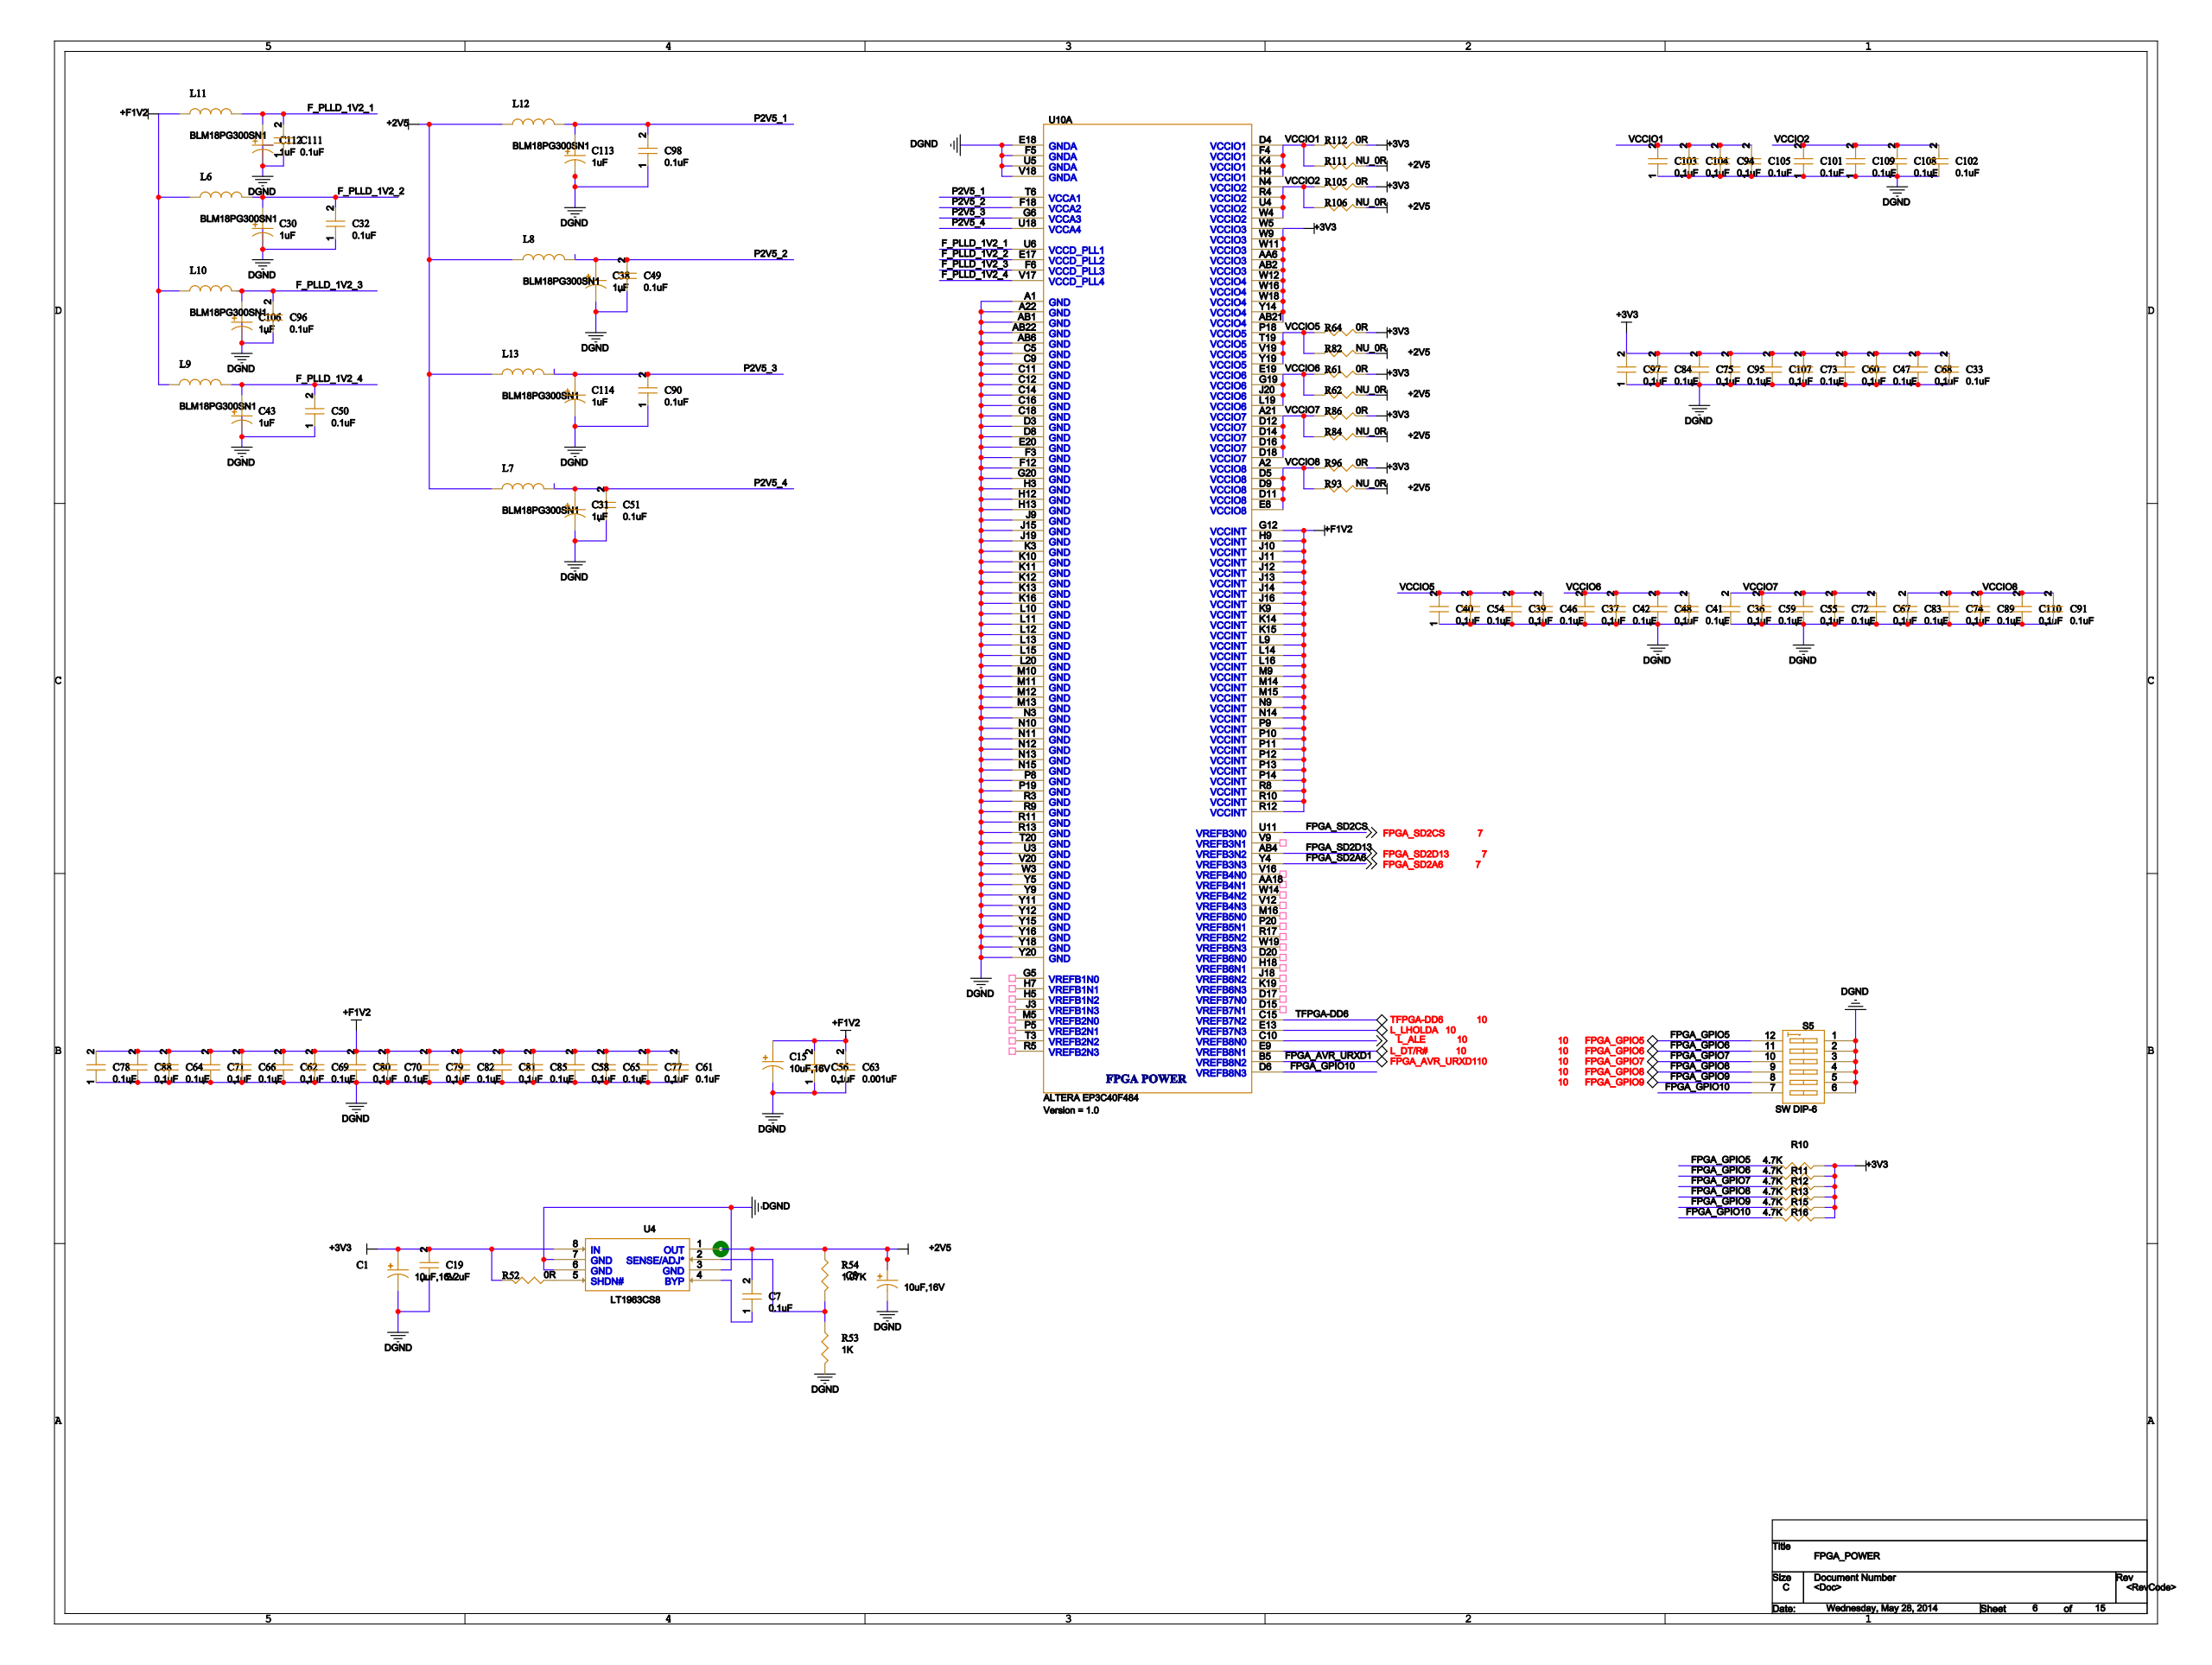Circuit board | Cadence Allegro | 669 parts | 806 nets | one sheet of the schematic
Parts on this sheet (reference | value | footprint):
C1 | 10uF,16V | CP3216
C14 | 10uF,16V | CP3216
C15 | 10uF,16V | CP3216
C19 | 2.2uF | C0603
C30 | 1uF | C0603
C31 | 1uF | C0603
C32 | 0.1uF | C0402-BGA
C33 | 0.1uF | C0402-BGA
C36 | 0.1uF | C0402-BGA
C37 | 0.1uF | C0402-BGA
C38 | 1uF | C0603
C39 | 0.1uF | C0402-BGA
C40 | 0.1uF | C0402-BGA
C41 | 0.1uF | C0402-BGA
C42 | 0.1uF | C0402-BGA
C43 | 1uF | C0603
C46 | 0.1uF | C0402-BGA
C47 | 0.1uF | C0402-BGA
C48 | 0.1uF | C0402-BGA
C49 | 0.1uF | C0402-BGA
C50 | 0.1uF | C0402-BGA
C51 | 0.1uF | C0402-BGA
C54 | 0.1uF | C0402-BGA
C55 | 0.1uF | C0402-BGA
C56 | 0.1uF | C0402-BGA
C58 | 0.1uF | C0402-BGA
C59 | 0.1uF | C0402-BGA
C60 | 0.1uF | C0402-BGA
C61 | 0.1uF | C0402-BGA
C62 | 0.1uF | C0402-BGA
C63 | 0.001uF | C0402
C64 | 0.1uF | C0402-BGA
C65 | 0.1uF | C0402-BGA
C66 | 0.1uF | C0402-BGA
C67 | 0.1uF | C0402-BGA
C68 | 0.1uF | C0402-BGA
C69 | 0.1uF | C0402-BGA
C70 | 0.1uF | C0402-BGA
C71 | 0.1uF | C0402-BGA
C72 | 0.1uF | C0402-BGA
C73 | 0.1uF | C0402-BGA
C74 | 0.1uF | C0402-BGA
C75 | 0.1uF | C0402-BGA
C77 | 0.1uF | C0402-BGA
C78 | 0.1uF | C0402-BGA
C79 | 0.1uF | C0402-BGA
C80 | 0.1uF | C0402-BGA
C81 | 0.1uF | C0402-BGA
C82 | 0.1uF | C0402-BGA
C83 | 0.1uF | C0402-BGA
C84 | 0.1uF | C0402-BGA
C85 | 0.1uF | C0402-BGA
C88 | 0.1uF | C0402-BGA
C89 | 0.1uF | C0402-BGA
C90 | 0.1uF | C0402-BGA
C91 | 0.1uF | C0402-BGA
C94 | 0.1uF | C0402-BGA
C95 | 0.1uF | C0402-BGA
C96 | 0.1uF | C0402-BGA
C97 | 0.1uF | C0402-BGA
C98 | 0.1uF | C0402-BGA
C101 | 0.1uF | C0402-BGA
C102 | 0.1uF | C0402-BGA
C103 | 0.1uF | C0402-BGA
C104 | 0.1uF | C0402-BGA
C105 | 0.1uF | C0402-BGA
C106 | 1uF | C0603
C107 | 0.1uF | C0402-BGA
C108 | 0.1uF | C0402-BGA
C109 | 0.1uF | C0402-BGA
C110 | 0.1uF | C0402-BGA
C111 | 0.1uF | C0402-BGA
C112 | 1uF | C0603
C113 | 1uF | C0603
C114 | 1uF | C0603
L6 | BLM18PG300SN1 | L0603
L7 | BLM18PG300SN1 | L0603
L8 | BLM18PG300SN1 | L0603
L9 | BLM18PG300SN1 | L0603
L10 | BLM18PG300SN1 | L0603
L11 | BLM18PG300SN1 | L0603
L12 | BLM18PG300SN1 | L0603
L13 | BLM18PG300SN1 | L0603
R10 | 4.7K | R0603
R11 | 4.7K | R0603
R12 | 4.7K | R0603
R13 | 4.7K | R0603
R15 | 4.7K | R0603
R16 | 4.7K | R0603
R52 | 0R | R0603
R53 | 1K | R0603
R54 | 1.07K | R0603
R61 | 0R | R0603
R62 | NU_0R | R0603
R64 | 0R | R0603
R82 | NU_0R | R0603
R84 | NU_0R | R0603
R86 | 0R | R0603
R93 | NU_0R | R0603
R96 | 0R | R0603
R105 | 0R | R0603
R106 | NU_0R | R0603
R111 | NU_0R | R0603
R112 | 0R | R0603
S5 | SW DIP-6 | SWITCH12
U4 | LT1963CS8 | SO8
U10 | EP3C40F484C8N | FBGA484
Nets of these parts (net: part-pin ...):
DGND: C1-2 C14-2 C15-2 C19-1 C30-2 C31-2 C32-1 C33-1 C36-1 C37-1 C38-2 C39-1 C40-1 C41-1 C42-1 C43-2 C46-1 C47-1 C48-1 C49-1 C50-1 C51-1 C54-1 C55-1 C56-1 C58-1 C59-1 C60-1 C61-1 C62-1 C63-1 C64-1 C65-1 C66-1 C67-1 C68-1 C69-1 C70-1 C71-1 C72-1 C73-1 C74-1 C75-1 C77-1 C78-1 C79-1 C80-1 C81-1 C82-1 C83-1 C84-1 C85-1 C88-1 C89-1 C90-1 C91-1 C94-1 C95-1 C96-1 C97-1 C98-1 C101-1 C102-1 C103-1 C104-1 C105-1 C106-2 C107-1 C108-1 C109-1 C110-1 C111-1 C112-2 C113-2 C114-2 R53-2 S5-1 S5-2 S5-3 S5-4 S5-5 S5-6 U4-3 U4-6 U4-7 U10-A1 U10-A22 U10-AB1 U10-AB6 U10-AB22 U10-C5 U10-C9 U10-C11 U10-C12 U10-C14 U10-C16 U10-C18 U10-D3 U10-D8 U10-E18 U10-E20 U10-F3 U10-F5 U10-F12 U10-G20 U10-H3 U10-H12 U10-H13 U10-J9 U10-J15 U10-J19 U10-K3 U10-K10 U10-K11 U10-K12 U10-K13 U10-K16 U10-L10 U10-L11 U10-L12 U10-L13 U10-L15 U10-L20 U10-M10 U10-M11 U10-M12 U10-M13 U10-N3 U10-N10 U10-N11 U10-N12 U10-N13 U10-N15 U10-P8 U10-P19 U10-R3 U10-R9 U10-R11 U10-R13 U10-T20 U10-U3 U10-U5 U10-V18 U10-V20 U10-W3 U10-Y5 U10-Y9 U10-Y11 U10-Y12 U10-Y15 U10-Y16 U10-Y18 U10-Y20
P2V5_1: C98-2 C113-1 L12-1 U10-T6
P2V5_2: C38-1 C49-2 L8-1 U10-F18
P2V5_3: C90-2 C114-1 L13-1 U10-G6
P2V5_4: C31-1 C51-2 L7-1 U10-U18
F_PLLD_1V2_1: C111-2 C112-1 L11-1 U10-U6
F_PLLD_1V2_2: C30-1 C32-2 L6-1 U10-E17
F_PLLD_1V2_3: C96-2 C106-1 L10-1 U10-F6
F_PLLD_1V2_4: C43-1 C50-2 L9-1 U10-V17
+F1V2: C15-1 C56-2 C58-2 C61-2 C62-2 C63-2 C64-2 C65-2 C66-2 C69-2 C70-2 C71-2 C77-2 C78-2 C79-2 C80-2 C81-2 C82-2 C85-2 C88-2 L6-2 L9-2 L10-2 L11-2 U10-G12 U10-H9 U10-J10 U10-J11 U10-J12 U10-J13 U10-J14 U10-J16 U10-K9 U10-K14 U10-K15 U10-L9 U10-L14 U10-L16 U10-M9 U10-M14 U10-M15 U10-N9 U10-N14 U10-P9 U10-P10 U10-P11 U10-P12 U10-P13 U10-P14 U10-R8 U10-R10 U10-R12
VCCIO1: C94-2 C103-2 C104-2 C105-2 R111-1 R112-1 U10-D4 U10-F4 U10-H4 U10-K4
VCCIO2: C101-2 C102-2 C108-2 C109-2 R105-1 R106-1 U10-N4 U10-R4 U10-U4 U10-W4
+3V3: C1-1 C14-1 C19-2 C33-2 C47-2 C60-2 C68-2 C73-2 C75-2 C84-2 C95-2 C97-2 C107-2 R10-2 R11-2 R12-2 R13-2 R15-2 R16-2 R52-2 R61-2 R64-2 R86-2 R96-2 R105-2 R112-2 U4-8 U10-AA6 U10-AB2 U10-AB21 U10-W5 U10-W9 U10-W11 U10-W12 U10-W16 U10-W18 U10-Y14
VCCIO5: C39-2 C40-2 C46-2 C54-2 R64-1 R82-1 U10-P18 U10-T19 U10-V19 U10-Y19
VCCIO6: C37-2 C41-2 C42-2 C48-2 R61-1 R62-1 U10-E19 U10-G19 U10-J20 U10-L19
VCCIO7: C36-2 C55-2 C59-2 C67-2 C72-2 R84-1 R86-1 U10-A21 U10-D12 U10-D14 U10-D16 U10-D18
VCCIO8: C74-2 C83-2 C89-2 C91-2 C110-2 R93-1 R96-1 U10-A2 U10-D5 U10-D9 U10-D11 U10-E8
FPGA_SD2CS: U10-U11
FPGA_SD2D13: U10-AB4
FPGA_SD2A6: U10-Y4
TFPGA-DD6: U10-C15
L_LHOLDA: U10-E13
L_ALE: U10-C10
L_DT/R#: U10-E9
FPGA_AVR_URXD1: U10-B5
FPGA_GPIO10: R16-1 S5-7 U10-D6
FPGA_GPIO8: R13-1 S5-9
FPGA_GPIO9: R15-1 S5-8
FPGA_GPIO7: R12-1 S5-10
FPGA_GPIO6: R11-1 S5-11
FPGA_GPIO5: R10-1 S5-12
+2V5: L7-2 L8-2 L12-2 L13-2 R54-1 R62-2 R82-2 R84-2 R93-2 R106-2 R111-2 U4-1
N361811100: R52-1 U4-5
N36181189: R53-1 R54-2 U4-2
N36181215: U4-4